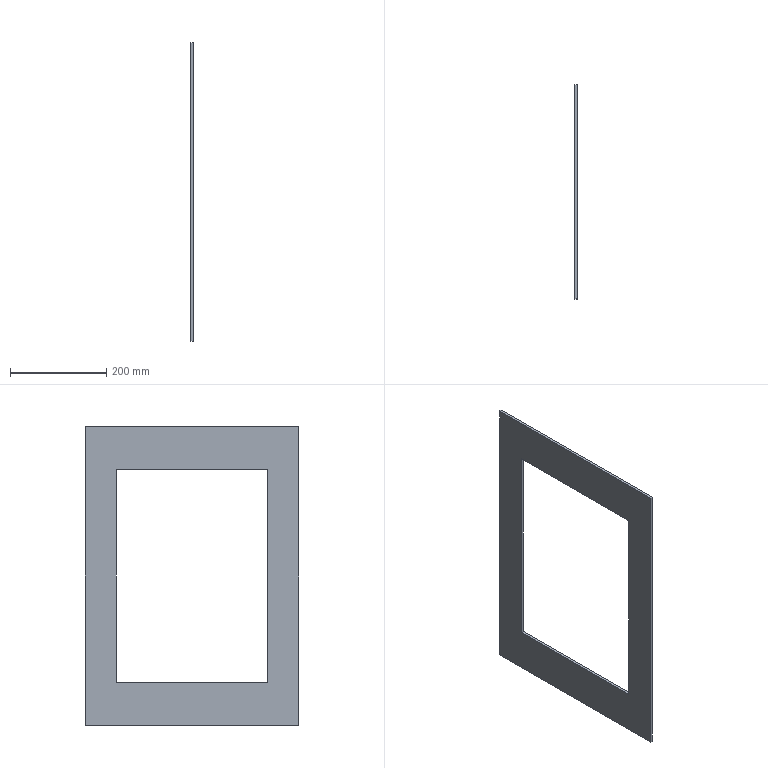Part | NX | features solid 2 | 1 solid | 10 faces | box 5 x 445 x 622 mm | volume 684010 mm3 | plane 10
STEP:
#1=CARTESIAN_POINT('',(2193.5,-893.5,883.));
#2=VERTEX_POINT('',#1);
#3=CARTESIAN_POINT('',(2188.5,-893.5,883.));
#4=VERTEX_POINT('',#3);
#5=CARTESIAN_POINT('',(2188.5,-893.5,883.));
#6=DIRECTION('',(-1.,0.,0.));
#7=VECTOR('',#6,1000.);
#8=LINE('',#5,#7);
#9=EDGE_CURVE('',#2,#4,#8,.T.);
#10=ORIENTED_EDGE('',*,*,#9,.T.);
#11=CARTESIAN_POINT('',(2188.5,-893.5,440.));
#12=VERTEX_POINT('',#11);
#13=CARTESIAN_POINT('',(2188.5,-893.5,972.5));
#14=DIRECTION('',(0.,0.,1.));
#15=VECTOR('',#14,1000.);
#16=LINE('',#13,#15);
#17=EDGE_CURVE('',#12,#4,#16,.T.);
#18=ORIENTED_EDGE('',*,*,#17,.F.);
#19=CARTESIAN_POINT('',(2193.5,-893.5,440.));
#20=VERTEX_POINT('',#19);
#21=CARTESIAN_POINT('',(2188.5,-893.5,440.));
#22=DIRECTION('',(-1.,0.,0.));
#23=VECTOR('',#22,1000.);
#24=LINE('',#21,#23);
#25=EDGE_CURVE('',#20,#12,#24,.T.);
#26=ORIENTED_EDGE('',*,*,#25,.F.);
#27=CARTESIAN_POINT('',(2193.5,-893.5,972.5));
#28=DIRECTION('',(0.,0.,1.));
#29=VECTOR('',#28,1000.);
#30=LINE('',#27,#29);
#31=EDGE_CURVE('',#20,#2,#30,.T.);
#32=ORIENTED_EDGE('',*,*,#31,.T.);
#33=EDGE_LOOP('',(#10,#18,#26,#32));
#34=FACE_BOUND('',#33,.T.);
#35=CARTESIAN_POINT('',(2188.5,-893.5,972.5));
#36=DIRECTION('',(0.,1.,0.));
#37=DIRECTION('',(0.,0.,-1.));
#38=AXIS2_PLACEMENT_3D('',#35,#36,#37);
#39=PLANE('',#38);
#40=ADVANCED_FACE('',(#34),#39,.F.);
#41=ORIENTED_EDGE('',*,*,#25,.T.);
#42=CARTESIAN_POINT('',(2188.5,-1209.5,440.));
#43=VERTEX_POINT('',#42);
#44=CARTESIAN_POINT('',(2188.5,-829.,440.));
#45=DIRECTION('',(0.,1.,0.));
#46=VECTOR('',#45,1000.);
#47=LINE('',#44,#46);
#48=EDGE_CURVE('',#43,#12,#47,.T.);
#49=ORIENTED_EDGE('',*,*,#48,.F.);
#50=CARTESIAN_POINT('',(2193.5,-1209.5,440.));
#51=VERTEX_POINT('',#50);
#52=CARTESIAN_POINT('',(2188.5,-1209.5,440.));
#53=DIRECTION('',(-1.,0.,0.));
#54=VECTOR('',#53,1000.);
#55=LINE('',#52,#54);
#56=EDGE_CURVE('',#51,#43,#55,.T.);
#57=ORIENTED_EDGE('',*,*,#56,.F.);
#58=CARTESIAN_POINT('',(2193.5,-829.,440.));
#59=DIRECTION('',(0.,1.,0.));
#60=VECTOR('',#59,1000.);
#61=LINE('',#58,#60);
#62=EDGE_CURVE('',#51,#20,#61,.T.);
#63=ORIENTED_EDGE('',*,*,#62,.T.);
#64=EDGE_LOOP('',(#41,#49,#57,#63));
#65=FACE_BOUND('',#64,.T.);
#66=CARTESIAN_POINT('',(2188.5,-829.,440.));
#67=DIRECTION('',(0.,0.,-1.));
#68=DIRECTION('',(0.,-1.,0.));
#69=AXIS2_PLACEMENT_3D('',#66,#67,#68);
#70=PLANE('',#69);
#71=ADVANCED_FACE('',(#65),#70,.F.);
#72=ORIENTED_EDGE('',*,*,#56,.T.);
#73=CARTESIAN_POINT('',(2188.5,-1209.5,883.));
#74=VERTEX_POINT('',#73);
#75=CARTESIAN_POINT('',(2188.5,-1209.5,972.5));
#76=DIRECTION('',(0.,0.,-1.));
#77=VECTOR('',#76,1000.);
#78=LINE('',#75,#77);
#79=EDGE_CURVE('',#74,#43,#78,.T.);
#80=ORIENTED_EDGE('',*,*,#79,.F.);
#81=CARTESIAN_POINT('',(2193.5,-1209.5,883.));
#82=VERTEX_POINT('',#81);
#83=CARTESIAN_POINT('',(2188.5,-1209.5,883.));
#84=DIRECTION('',(-1.,0.,0.));
#85=VECTOR('',#84,1000.);
#86=LINE('',#83,#85);
#87=EDGE_CURVE('',#82,#74,#86,.T.);
#88=ORIENTED_EDGE('',*,*,#87,.F.);
#89=CARTESIAN_POINT('',(2193.5,-1209.5,972.5));
#90=DIRECTION('',(0.,0.,-1.));
#91=VECTOR('',#90,1000.);
#92=LINE('',#89,#91);
#93=EDGE_CURVE('',#82,#51,#92,.T.);
#94=ORIENTED_EDGE('',*,*,#93,.T.);
#95=EDGE_LOOP('',(#72,#80,#88,#94));
#96=FACE_BOUND('',#95,.T.);
#97=CARTESIAN_POINT('',(2188.5,-1209.5,972.5));
#98=DIRECTION('',(0.,-1.,0.));
#99=DIRECTION('',(-1.,0.,0.));
#100=AXIS2_PLACEMENT_3D('',#97,#98,#99);
#101=PLANE('',#100);
#102=ADVANCED_FACE('',(#96),#101,.F.);
#103=CARTESIAN_POINT('',(2193.5,-829.,883.));
#104=DIRECTION('',(0.,-1.,0.));
#105=VECTOR('',#104,1000.);
#106=LINE('',#103,#105);
#107=EDGE_CURVE('',#2,#82,#106,.T.);
#108=ORIENTED_EDGE('',*,*,#107,.T.);
#109=ORIENTED_EDGE('',*,*,#87,.T.);
#110=CARTESIAN_POINT('',(2188.5,-829.,883.));
#111=DIRECTION('',(0.,-1.,0.));
#112=VECTOR('',#111,1000.);
#113=LINE('',#110,#112);
#114=EDGE_CURVE('',#4,#74,#113,.T.);
#115=ORIENTED_EDGE('',*,*,#114,.F.);
#116=ORIENTED_EDGE('',*,*,#9,.F.);
#117=EDGE_LOOP('',(#108,#109,#115,#116));
#118=FACE_BOUND('',#117,.T.);
#119=CARTESIAN_POINT('',(2188.5,-829.,883.));
#120=DIRECTION('',(0.,0.,1.));
#121=DIRECTION('',(0.,-1.,0.));
#122=AXIS2_PLACEMENT_3D('',#119,#120,#121);
#123=PLANE('',#122);
#124=ADVANCED_FACE('',(#118),#123,.F.);
#125=ORIENTED_EDGE('',*,*,#48,.T.);
#126=ORIENTED_EDGE('',*,*,#17,.T.);
#127=ORIENTED_EDGE('',*,*,#114,.T.);
#128=ORIENTED_EDGE('',*,*,#79,.T.);
#129=EDGE_LOOP('',(#125,#126,#127,#128));
#130=FACE_BOUND('',#129,.T.);
#131=CARTESIAN_POINT('',(2188.5,-829.,350.5));
#132=VERTEX_POINT('',#131);
#133=CARTESIAN_POINT('',(2188.5,-829.,972.5));
#134=VERTEX_POINT('',#133);
#135=CARTESIAN_POINT('',(2188.5,-829.,350.5));
#136=DIRECTION('',(0.,0.,1.));
#137=VECTOR('',#136,1000.);
#138=LINE('',#135,#137);
#139=EDGE_CURVE('',#132,#134,#138,.T.);
#140=ORIENTED_EDGE('',*,*,#139,.F.);
#141=CARTESIAN_POINT('',(2188.5,-1274.,350.5));
#142=VERTEX_POINT('',#141);
#143=CARTESIAN_POINT('',(2188.5,-1274.,350.5));
#144=DIRECTION('',(0.,1.,0.));
#145=VECTOR('',#144,1000.);
#146=LINE('',#143,#145);
#147=EDGE_CURVE('',#142,#132,#146,.T.);
#148=ORIENTED_EDGE('',*,*,#147,.F.);
#149=CARTESIAN_POINT('',(2188.5,-1274.,972.5));
#150=VERTEX_POINT('',#149);
#151=CARTESIAN_POINT('',(2188.5,-1274.,972.5));
#152=DIRECTION('',(0.,0.,-1.));
#153=VECTOR('',#152,1000.);
#154=LINE('',#151,#153);
#155=EDGE_CURVE('',#150,#142,#154,.T.);
#156=ORIENTED_EDGE('',*,*,#155,.F.);
#157=CARTESIAN_POINT('',(2188.5,-829.,972.5));
#158=DIRECTION('',(0.,-1.,0.));
#159=VECTOR('',#158,1000.);
#160=LINE('',#157,#159);
#161=EDGE_CURVE('',#134,#150,#160,.T.);
#162=ORIENTED_EDGE('',*,*,#161,.F.);
#163=EDGE_LOOP('',(#140,#148,#156,#162));
#164=FACE_BOUND('',#163,.T.);
#165=CARTESIAN_POINT('',(2188.5,-829.,972.5));
#166=DIRECTION('',(1.,0.,0.));
#167=DIRECTION('',(0.,0.,-1.));
#168=AXIS2_PLACEMENT_3D('',#165,#166,#167);
#169=PLANE('',#168);
#170=ADVANCED_FACE('',(#130,#164),#169,.F.);
#171=ORIENTED_EDGE('',*,*,#31,.F.);
#172=ORIENTED_EDGE('',*,*,#62,.F.);
#173=ORIENTED_EDGE('',*,*,#93,.F.);
#174=ORIENTED_EDGE('',*,*,#107,.F.);
#175=EDGE_LOOP('',(#171,#172,#173,#174));
#176=FACE_BOUND('',#175,.T.);
#177=CARTESIAN_POINT('',(2193.5,-829.,350.5));
#178=VERTEX_POINT('',#177);
#179=CARTESIAN_POINT('',(2193.5,-829.,972.5));
#180=VERTEX_POINT('',#179);
#181=CARTESIAN_POINT('',(2193.5,-829.,350.5));
#182=DIRECTION('',(0.,0.,1.));
#183=VECTOR('',#182,1000.);
#184=LINE('',#181,#183);
#185=EDGE_CURVE('',#178,#180,#184,.T.);
#186=ORIENTED_EDGE('',*,*,#185,.T.);
#187=CARTESIAN_POINT('',(2193.5,-1274.,972.5));
#188=VERTEX_POINT('',#187);
#189=CARTESIAN_POINT('',(2193.5,-829.,972.5));
#190=DIRECTION('',(0.,-1.,0.));
#191=VECTOR('',#190,1000.);
#192=LINE('',#189,#191);
#193=EDGE_CURVE('',#180,#188,#192,.T.);
#194=ORIENTED_EDGE('',*,*,#193,.T.);
#195=CARTESIAN_POINT('',(2193.5,-1274.,350.5));
#196=VERTEX_POINT('',#195);
#197=CARTESIAN_POINT('',(2193.5,-1274.,972.5));
#198=DIRECTION('',(0.,0.,-1.));
#199=VECTOR('',#198,1000.);
#200=LINE('',#197,#199);
#201=EDGE_CURVE('',#188,#196,#200,.T.);
#202=ORIENTED_EDGE('',*,*,#201,.T.);
#203=CARTESIAN_POINT('',(2193.5,-1274.,350.5));
#204=DIRECTION('',(0.,1.,0.));
#205=VECTOR('',#204,1000.);
#206=LINE('',#203,#205);
#207=EDGE_CURVE('',#196,#178,#206,.T.);
#208=ORIENTED_EDGE('',*,*,#207,.T.);
#209=EDGE_LOOP('',(#186,#194,#202,#208));
#210=FACE_BOUND('',#209,.T.);
#211=CARTESIAN_POINT('',(2193.5,-829.,972.5));
#212=DIRECTION('',(1.,0.,0.));
#213=DIRECTION('',(0.,0.,-1.));
#214=AXIS2_PLACEMENT_3D('',#211,#212,#213);
#215=PLANE('',#214);
#216=ADVANCED_FACE('',(#176,#210),#215,.T.);
#217=ORIENTED_EDGE('',*,*,#147,.T.);
#218=CARTESIAN_POINT('',(2193.5,-829.,350.5));
#219=DIRECTION('',(-1.,0.,0.));
#220=VECTOR('',#219,1000.);
#221=LINE('',#218,#220);
#222=EDGE_CURVE('',#178,#132,#221,.T.);
#223=ORIENTED_EDGE('',*,*,#222,.F.);
#224=ORIENTED_EDGE('',*,*,#207,.F.);
#225=CARTESIAN_POINT('',(2193.5,-1274.,350.5));
#226=DIRECTION('',(-1.,0.,0.));
#227=VECTOR('',#226,1000.);
#228=LINE('',#225,#227);
#229=EDGE_CURVE('',#196,#142,#228,.T.);
#230=ORIENTED_EDGE('',*,*,#229,.T.);
#231=EDGE_LOOP('',(#217,#223,#224,#230));
#232=FACE_BOUND('',#231,.T.);
#233=CARTESIAN_POINT('',(2193.5,-1274.,350.5));
#234=DIRECTION('',(0.,0.,1.));
#235=DIRECTION('',(0.,-1.,0.));
#236=AXIS2_PLACEMENT_3D('',#233,#234,#235);
#237=PLANE('',#236);
#238=ADVANCED_FACE('',(#232),#237,.F.);
#239=ORIENTED_EDGE('',*,*,#155,.T.);
#240=ORIENTED_EDGE('',*,*,#229,.F.);
#241=ORIENTED_EDGE('',*,*,#201,.F.);
#242=CARTESIAN_POINT('',(2193.5,-1274.,972.5));
#243=DIRECTION('',(-1.,0.,0.));
#244=VECTOR('',#243,1000.);
#245=LINE('',#242,#244);
#246=EDGE_CURVE('',#188,#150,#245,.T.);
#247=ORIENTED_EDGE('',*,*,#246,.T.);
#248=EDGE_LOOP('',(#239,#240,#241,#247));
#249=FACE_BOUND('',#248,.T.);
#250=CARTESIAN_POINT('',(2193.5,-1274.,972.5));
#251=DIRECTION('',(0.,1.,0.));
#252=DIRECTION('',(0.,0.,-1.));
#253=AXIS2_PLACEMENT_3D('',#250,#251,#252);
#254=PLANE('',#253);
#255=ADVANCED_FACE('',(#249),#254,.F.);
#256=ORIENTED_EDGE('',*,*,#161,.T.);
#257=ORIENTED_EDGE('',*,*,#246,.F.);
#258=ORIENTED_EDGE('',*,*,#193,.F.);
#259=CARTESIAN_POINT('',(2193.5,-829.,972.5));
#260=DIRECTION('',(-1.,0.,0.));
#261=VECTOR('',#260,1000.);
#262=LINE('',#259,#261);
#263=EDGE_CURVE('',#180,#134,#262,.T.);
#264=ORIENTED_EDGE('',*,*,#263,.T.);
#265=EDGE_LOOP('',(#256,#257,#258,#264));
#266=FACE_BOUND('',#265,.T.);
#267=CARTESIAN_POINT('',(2193.5,-829.,972.5));
#268=DIRECTION('',(0.,0.,-1.));
#269=DIRECTION('',(0.,-1.,0.));
#270=AXIS2_PLACEMENT_3D('',#267,#268,#269);
#271=PLANE('',#270);
#272=ADVANCED_FACE('',(#266),#271,.F.);
#273=ORIENTED_EDGE('',*,*,#139,.T.);
#274=ORIENTED_EDGE('',*,*,#263,.F.);
#275=ORIENTED_EDGE('',*,*,#185,.F.);
#276=ORIENTED_EDGE('',*,*,#222,.T.);
#277=EDGE_LOOP('',(#273,#274,#275,#276));
#278=FACE_BOUND('',#277,.T.);
#279=CARTESIAN_POINT('',(2193.5,-829.,350.5));
#280=DIRECTION('',(0.,-1.,0.));
#281=DIRECTION('',(-1.,0.,0.));
#282=AXIS2_PLACEMENT_3D('',#279,#280,#281);
#283=PLANE('',#282);
#284=ADVANCED_FACE('',(#278),#283,.F.);
#285=CLOSED_SHELL('',(#40,#71,#102,#124,#170,#216,#238,#255,#272,#284));
#286=MANIFOLD_SOLID_BREP('',#285);
#287=(LENGTH_UNIT()NAMED_UNIT(*)SI_UNIT(.MILLI.,.METRE.));
#288=UNCERTAINTY_MEASURE_WITH_UNIT(LENGTH_MEASURE(0.00001),#287,'','');
#289=(NAMED_UNIT(*)PLANE_ANGLE_UNIT()SI_UNIT($,.RADIAN.));
#290=(NAMED_UNIT(*)SI_UNIT($,.STERADIAN.)SOLID_ANGLE_UNIT());
#291=(GEOMETRIC_REPRESENTATION_CONTEXT(3)GLOBAL_UNCERTAINTY_ASSIGNED_CONTEXT((#288))GLOBAL_UNIT_ASSIGNED_CONTEXT((#287,#289,#290))REPRESENTATION_CONTEXT('',''));
#292=ADVANCED_BREP_SHAPE_REPRESENTATION('',(#286),#291);